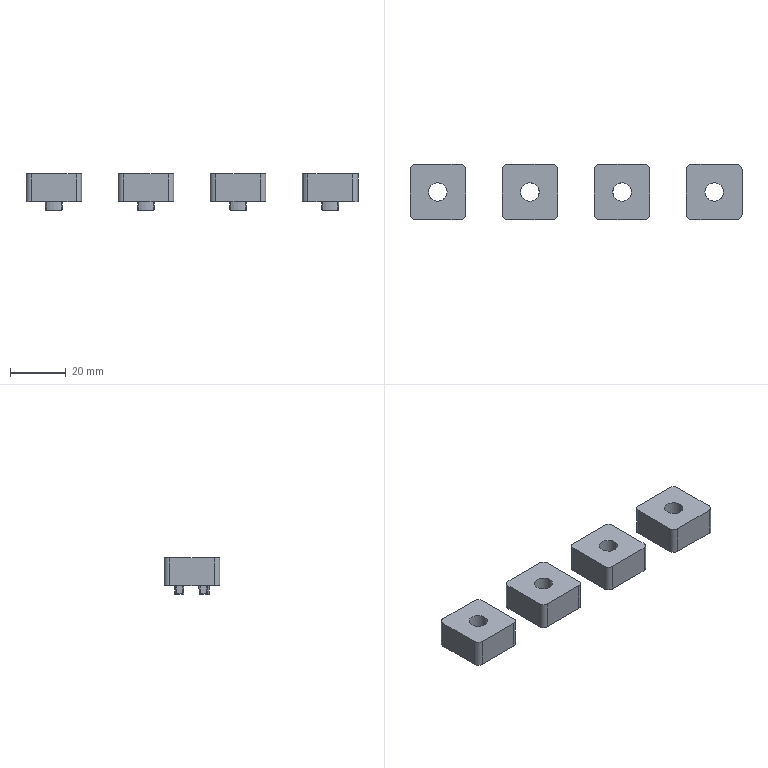NC program | NX | posted with a generic post | part box 118.91 x 19.91 x 13 mm
Lines 19 to 871 of 17620:
(ZLEVEL_PROFILE , TOOL : D10)
N36 T15 M6
N38 G54
N40 G17 G0 G90 X34.445 Y6.508 S9500 M3
N42 G43 Z30. H15
N44 Z1.5
N46 G94 G1 Y8.651 Z1.388 F1000.
N48 X34.782 Y10.25 Z1.302
N50 X35.476 Y11.729 Z1.216
N52 X36.49 Y13.01 Z1.131
N54 X37.771 Y14.024 Z1.045
N56 X39.25 Y14.718 Z0.96
N58 X40.849 Y15.055 Z0.874
N60 X58.151 Z-0.033
N62 X59.75 Y14.718 Z-0.118
N64 X61.229 Y14.024 Z-0.204
N66 X62.51 Y13.01 Z-0.29
N68 X63.524 Y11.729 Z-0.375
N70 X64.218 Y10.25 Z-0.461
N72 X64.555 Y8.651 Z-0.547
N74 Y0. Z-1.
N76 Y-8. F3000.
N78 G2 X57.5 Y-15.055 R7.055
N80 G1 X41.5
N82 G2 X34.445 Y-8. R7.055
N84 G1 Y8.
N86 G2 X41.5 Y15.055 R7.055
N88 G1 X57.5
N90 G2 X64.555 Y8. R7.055
N92 G1 Y0.
N94 Y-8. Z-1.074
N96 X64.528 Y-8.615 Z-1.08
N98 X64.448 Y-9.225 Z-1.085
N100 X64.315 Y-9.826 Z-1.091
N102 X64.13 Y-10.413 Z-1.097
N104 X63.894 Y-10.982 Z-1.102
N106 X63.61 Y-11.528 Z-1.108
N108 X63.279 Y-12.047 Z-1.114
N110 X62.904 Y-12.535 Z-1.119
N112 X62.489 Y-12.989 Z-1.125
N114 X62.035 Y-13.404 Z-1.131
N116 X61.547 Y-13.779 Z-1.136
N118 X61.028 Y-14.11 Z-1.142
N120 X60.482 Y-14.394 Z-1.148
N122 X59.913 Y-14.63 Z-1.153
N124 X59.326 Y-14.815 Z-1.159
N126 X58.725 Y-14.948 Z-1.165
N128 X58.115 Y-15.028 Z-1.17
N130 X57.5 Y-15.055 Z-1.176
N132 X41.5 Z-1.324
N134 X40.885 Y-15.028 Z-1.33
N136 X40.275 Y-14.948 Z-1.335
N138 X39.674 Y-14.815 Z-1.341
N140 X39.087 Y-14.63 Z-1.347
N142 X38.518 Y-14.394 Z-1.352
N144 X37.973 Y-14.11 Z-1.358
N146 X37.453 Y-13.779 Z-1.364
N148 X36.965 Y-13.404 Z-1.369
N150 X36.511 Y-12.989 Z-1.375
N152 X36.096 Y-12.535 Z-1.381
N154 X35.721 Y-12.047 Z-1.386
N156 X35.39 Y-11.528 Z-1.392
N158 X35.106 Y-10.982 Z-1.398
N160 X34.87 Y-10.413 Z-1.403
N162 X34.685 Y-9.826 Z-1.409
N164 X34.552 Y-9.225 Z-1.415
N166 X34.472 Y-8.615 Z-1.42
N168 X34.445 Y-8. Z-1.426
N170 Y0. Z-1.5
N172 Y4. Z-1.537
N174 Y8. Z-1.574
N176 X34.472 Y8.615 Z-1.58
N178 X34.552 Y9.225 Z-1.585
N180 X34.685 Y9.826 Z-1.591
N182 X34.87 Y10.413 Z-1.597
N184 X35.106 Y10.982 Z-1.602
N186 X35.39 Y11.528 Z-1.608
N188 X35.721 Y12.047 Z-1.614
N190 X36.096 Y12.535 Z-1.619
N192 X36.511 Y12.989 Z-1.625
N194 X36.965 Y13.404 Z-1.631
N196 X37.453 Y13.779 Z-1.636
N198 X37.973 Y14.11 Z-1.642
N200 X38.518 Y14.394 Z-1.648
N202 X39.087 Y14.63 Z-1.653
N204 X39.674 Y14.815 Z-1.659
N206 X40.275 Y14.948 Z-1.665
N208 X40.885 Y15.028 Z-1.67
N210 X41.5 Y15.055 Z-1.676
N212 X57.5 Z-1.824
N214 X58.115 Y15.028 Z-1.83
N216 X58.725 Y14.948 Z-1.835
N218 X59.326 Y14.815 Z-1.841
N220 X59.913 Y14.63 Z-1.847
N222 X60.482 Y14.394 Z-1.852
N224 X61.028 Y14.11 Z-1.858
N226 X61.547 Y13.779 Z-1.864
N228 X62.035 Y13.404 Z-1.869
N230 X62.489 Y12.989 Z-1.875
N232 X62.904 Y12.535 Z-1.881
N234 X63.279 Y12.047 Z-1.886
N236 X63.61 Y11.528 Z-1.892
N238 X63.894 Y10.982 Z-1.898
N240 X64.13 Y10.413 Z-1.903
N242 X64.315 Y9.826 Z-1.909
N244 X64.448 Y9.225 Z-1.915
N246 X64.528 Y8.615 Z-1.92
N248 X64.555 Y8. Z-1.926
N250 Y0. Z-2.
N252 Y-8. Z-2.074
N254 X64.528 Y-8.615 Z-2.08
N256 X64.448 Y-9.225 Z-2.085
N258 X64.315 Y-9.826 Z-2.091
N260 X64.13 Y-10.413 Z-2.097
N262 X63.894 Y-10.982 Z-2.102
N264 X63.61 Y-11.528 Z-2.108
N266 X63.279 Y-12.047 Z-2.114
N268 X62.904 Y-12.535 Z-2.119
N270 X62.489 Y-12.989 Z-2.125
N272 X62.035 Y-13.404 Z-2.131
N274 X61.547 Y-13.779 Z-2.136
N276 X61.028 Y-14.11 Z-2.142
N278 X60.482 Y-14.394 Z-2.148
N280 X59.913 Y-14.63 Z-2.153
N282 X59.326 Y-14.815 Z-2.159
N284 X58.725 Y-14.948 Z-2.165
N286 X58.115 Y-15.028 Z-2.17
N288 X57.5 Y-15.055 Z-2.176
N290 X41.5 Z-2.324
N292 X40.885 Y-15.028 Z-2.33
N294 X40.275 Y-14.948 Z-2.335
N296 X39.674 Y-14.815 Z-2.341
N298 X39.087 Y-14.63 Z-2.347
N300 X38.518 Y-14.394 Z-2.352
N302 X37.973 Y-14.11 Z-2.358
N304 X37.453 Y-13.779 Z-2.364
N306 X36.965 Y-13.404 Z-2.369
N308 X36.511 Y-12.989 Z-2.375
N310 X36.096 Y-12.535 Z-2.381
N312 X35.721 Y-12.047 Z-2.386
N314 X35.39 Y-11.528 Z-2.392
N316 X35.106 Y-10.982 Z-2.398
N318 X34.87 Y-10.413 Z-2.403
N320 X34.685 Y-9.826 Z-2.409
N322 X34.552 Y-9.225 Z-2.415
N324 X34.472 Y-8.615 Z-2.42
N326 X34.445 Y-8. Z-2.426
N328 Y0. Z-2.5
N330 Y4. Z-2.537
N332 Y8. Z-2.574
N334 X34.472 Y8.615 Z-2.58
N336 X34.552 Y9.225 Z-2.585
N338 X34.685 Y9.826 Z-2.591
N340 X34.87 Y10.413 Z-2.597
N342 X35.106 Y10.982 Z-2.602
N344 X35.39 Y11.528 Z-2.608
N346 X35.721 Y12.047 Z-2.614
N348 X36.096 Y12.535 Z-2.619
N350 X36.511 Y12.989 Z-2.625
N352 X36.965 Y13.404 Z-2.631
N354 X37.453 Y13.779 Z-2.636
N356 X37.973 Y14.11 Z-2.642
N358 X38.518 Y14.394 Z-2.648
N360 X39.087 Y14.63 Z-2.653
N362 X39.674 Y14.815 Z-2.659
N364 X40.275 Y14.948 Z-2.665
N366 X40.885 Y15.028 Z-2.67
N368 X41.5 Y15.055 Z-2.676
N370 X57.5 Z-2.824
N372 X58.115 Y15.028 Z-2.83
N374 X58.725 Y14.948 Z-2.835
N376 X59.326 Y14.815 Z-2.841
N378 X59.913 Y14.63 Z-2.847
N380 X60.482 Y14.394 Z-2.852
N382 X61.028 Y14.11 Z-2.858
N384 X61.547 Y13.779 Z-2.864
N386 X62.035 Y13.404 Z-2.869
N388 X62.489 Y12.989 Z-2.875
N390 X62.904 Y12.535 Z-2.881
N392 X63.279 Y12.047 Z-2.886
N394 X63.61 Y11.528 Z-2.892
N396 X63.894 Y10.982 Z-2.898
N398 X64.13 Y10.413 Z-2.903
N400 X64.315 Y9.826 Z-2.909
N402 X64.448 Y9.225 Z-2.915
N404 X64.528 Y8.615 Z-2.92
N406 X64.555 Y8. Z-2.926
N408 Y0. Z-3.
N410 Y-8. Z-3.074
N412 X64.528 Y-8.615 Z-3.08
N414 X64.448 Y-9.225 Z-3.085
N416 X64.315 Y-9.826 Z-3.091
N418 X64.13 Y-10.413 Z-3.097
N420 X63.894 Y-10.982 Z-3.102
N422 X63.61 Y-11.528 Z-3.108
N424 X63.279 Y-12.047 Z-3.114
N426 X62.904 Y-12.535 Z-3.119
N428 X62.489 Y-12.989 Z-3.125
N430 X62.035 Y-13.404 Z-3.131
N432 X61.547 Y-13.779 Z-3.136
N434 X61.028 Y-14.11 Z-3.142
N436 X60.482 Y-14.394 Z-3.148
N438 X59.913 Y-14.63 Z-3.153
N440 X59.326 Y-14.815 Z-3.159
N442 X58.725 Y-14.948 Z-3.165
N444 X58.115 Y-15.028 Z-3.17
N446 X57.5 Y-15.055 Z-3.176
N448 X41.5 Z-3.324
N450 X40.885 Y-15.028 Z-3.33
N452 X40.275 Y-14.948 Z-3.335
N454 X39.674 Y-14.815 Z-3.341
N456 X39.087 Y-14.63 Z-3.347
N458 X38.518 Y-14.394 Z-3.352
N460 X37.973 Y-14.11 Z-3.358
N462 X37.453 Y-13.779 Z-3.364
N464 X36.965 Y-13.404 Z-3.369
N466 X36.511 Y-12.989 Z-3.375
N468 X36.096 Y-12.535 Z-3.381
N470 X35.721 Y-12.047 Z-3.386
N472 X35.39 Y-11.528 Z-3.392
N474 X35.106 Y-10.982 Z-3.398
N476 X34.87 Y-10.413 Z-3.403
N478 X34.685 Y-9.826 Z-3.409
N480 X34.552 Y-9.225 Z-3.415
N482 X34.472 Y-8.615 Z-3.42
N484 X34.445 Y-8. Z-3.426
N486 Y0. Z-3.5
N488 Y4. Z-3.537
N490 Y8. Z-3.574
N492 X34.472 Y8.615 Z-3.58
N494 X34.552 Y9.225 Z-3.585
N496 X34.685 Y9.826 Z-3.591
N498 X34.87 Y10.413 Z-3.597
N500 X35.106 Y10.982 Z-3.602
N502 X35.39 Y11.528 Z-3.608
N504 X35.721 Y12.047 Z-3.614
N506 X36.096 Y12.535 Z-3.619
N508 X36.511 Y12.989 Z-3.625
N510 X36.965 Y13.404 Z-3.631
N512 X37.453 Y13.779 Z-3.636
N514 X37.973 Y14.11 Z-3.642
N516 X38.518 Y14.394 Z-3.648
N518 X39.087 Y14.63 Z-3.653
N520 X39.674 Y14.815 Z-3.659
N522 X40.275 Y14.948 Z-3.665
N524 X40.885 Y15.028 Z-3.67
N526 X41.5 Y15.055 Z-3.676
N528 X57.5 Z-3.824
N530 X58.115 Y15.028 Z-3.83
N532 X58.725 Y14.948 Z-3.835
N534 X59.326 Y14.815 Z-3.841
N536 X59.913 Y14.63 Z-3.847
N538 X60.482 Y14.394 Z-3.852
N540 X61.028 Y14.11 Z-3.858
N542 X61.547 Y13.779 Z-3.864
N544 X62.035 Y13.404 Z-3.869
N546 X62.489 Y12.989 Z-3.875
N548 X62.904 Y12.535 Z-3.881
N550 X63.279 Y12.047 Z-3.886
N552 X63.61 Y11.528 Z-3.892
N554 X63.894 Y10.982 Z-3.898
N556 X64.13 Y10.413 Z-3.903
N558 X64.315 Y9.826 Z-3.909
N560 X64.448 Y9.225 Z-3.915
N562 X64.528 Y8.615 Z-3.92
N564 X64.555 Y8. Z-3.926
N566 Y0. Z-4.
N568 Y-8. Z-4.074
N570 X64.528 Y-8.615 Z-4.08
N572 X64.448 Y-9.225 Z-4.085
N574 X64.315 Y-9.826 Z-4.091
N576 X64.13 Y-10.413 Z-4.097
N578 X63.894 Y-10.982 Z-4.102
N580 X63.61 Y-11.528 Z-4.108
N582 X63.279 Y-12.047 Z-4.114
N584 X62.904 Y-12.535 Z-4.119
N586 X62.489 Y-12.989 Z-4.125
N588 X62.035 Y-13.404 Z-4.131
N590 X61.547 Y-13.779 Z-4.136
N592 X61.028 Y-14.11 Z-4.142
N594 X60.482 Y-14.394 Z-4.148
N596 X59.913 Y-14.63 Z-4.153
N598 X59.326 Y-14.815 Z-4.159
N600 X58.725 Y-14.948 Z-4.165
N602 X58.115 Y-15.028 Z-4.17
N604 X57.5 Y-15.055 Z-4.176
N606 X41.5 Z-4.324
N608 X40.885 Y-15.028 Z-4.33
N610 X40.275 Y-14.948 Z-4.335
N612 X39.674 Y-14.815 Z-4.341
N614 X39.087 Y-14.63 Z-4.347
N616 X38.518 Y-14.394 Z-4.352
N618 X37.973 Y-14.11 Z-4.358
N620 X37.453 Y-13.779 Z-4.364
N622 X36.965 Y-13.404 Z-4.369
N624 X36.511 Y-12.989 Z-4.375
N626 X36.096 Y-12.535 Z-4.381
N628 X35.721 Y-12.047 Z-4.386
N630 X35.39 Y-11.528 Z-4.392
N632 X35.106 Y-10.982 Z-4.398
N634 X34.87 Y-10.413 Z-4.403
N636 X34.685 Y-9.826 Z-4.409
N638 X34.552 Y-9.225 Z-4.415
N640 X34.472 Y-8.615 Z-4.42
N642 X34.445 Y-8. Z-4.426
N644 Y0. Z-4.5
N646 Y4. Z-4.537
N648 Y8. Z-4.574
N650 X34.472 Y8.615 Z-4.58
N652 X34.552 Y9.225 Z-4.585
N654 X34.685 Y9.826 Z-4.591
N656 X34.87 Y10.413 Z-4.597
N658 X35.106 Y10.982 Z-4.602
N660 X35.39 Y11.528 Z-4.608
N662 X35.721 Y12.047 Z-4.614
N664 X36.096 Y12.535 Z-4.619
N666 X36.511 Y12.989 Z-4.625
N668 X36.965 Y13.404 Z-4.631
N670 X37.453 Y13.779 Z-4.636
N672 X37.973 Y14.11 Z-4.642
N674 X38.518 Y14.394 Z-4.648
N676 X39.087 Y14.63 Z-4.653
N678 X39.674 Y14.815 Z-4.659
N680 X40.275 Y14.948 Z-4.665
N682 X40.885 Y15.028 Z-4.67
N684 X41.5 Y15.055 Z-4.676
N686 X57.5 Z-4.824
N688 X58.115 Y15.028 Z-4.83
N690 X58.725 Y14.948 Z-4.835
N692 X59.326 Y14.815 Z-4.841
N694 X59.913 Y14.63 Z-4.847
N696 X60.482 Y14.394 Z-4.852
N698 X61.028 Y14.11 Z-4.858
N700 X61.547 Y13.779 Z-4.864
N702 X62.035 Y13.404 Z-4.869
N704 X62.489 Y12.989 Z-4.875
N706 X62.904 Y12.535 Z-4.881
N708 X63.279 Y12.047 Z-4.886
N710 X63.61 Y11.528 Z-4.892
N712 X63.894 Y10.982 Z-4.898
N714 X64.13 Y10.413 Z-4.903
N716 X64.315 Y9.826 Z-4.909
N718 X64.448 Y9.225 Z-4.915
N720 X64.528 Y8.615 Z-4.92
N722 X64.555 Y8. Z-4.926
N724 Y0. Z-5.
N726 Y-8. Z-5.074
N728 X64.528 Y-8.615 Z-5.08
N730 X64.448 Y-9.225 Z-5.085
N732 X64.315 Y-9.826 Z-5.091
N734 X64.13 Y-10.413 Z-5.097
N736 X63.894 Y-10.982 Z-5.102
N738 X63.61 Y-11.528 Z-5.108
N740 X63.279 Y-12.047 Z-5.114
N742 X62.904 Y-12.535 Z-5.119
N744 X62.489 Y-12.989 Z-5.125
N746 X62.035 Y-13.404 Z-5.131
N748 X61.547 Y-13.779 Z-5.136
N750 X61.028 Y-14.11 Z-5.142
N752 X60.482 Y-14.394 Z-5.148
N754 X59.913 Y-14.63 Z-5.153
N756 X59.326 Y-14.815 Z-5.159
N758 X58.725 Y-14.948 Z-5.165
N760 X58.115 Y-15.028 Z-5.17
N762 X57.5 Y-15.055 Z-5.176
N764 X41.5 Z-5.324
N766 X40.885 Y-15.028 Z-5.33
N768 X40.275 Y-14.948 Z-5.335
N770 X39.674 Y-14.815 Z-5.341
N772 X39.087 Y-14.63 Z-5.347
N774 X38.518 Y-14.394 Z-5.352
N776 X37.973 Y-14.11 Z-5.358
N778 X37.453 Y-13.779 Z-5.364
N780 X36.965 Y-13.404 Z-5.369
N782 X36.511 Y-12.989 Z-5.375
N784 X36.096 Y-12.535 Z-5.381
N786 X35.721 Y-12.047 Z-5.386
N788 X35.39 Y-11.528 Z-5.392
N790 X35.106 Y-10.982 Z-5.398
N792 X34.87 Y-10.413 Z-5.403
N794 X34.685 Y-9.826 Z-5.409
N796 X34.552 Y-9.225 Z-5.415
N798 X34.472 Y-8.615 Z-5.42
N800 X34.445 Y-8. Z-5.426
N802 Y0. Z-5.5
N804 Y4. Z-5.537
N806 Y8. Z-5.574
N808 X34.472 Y8.615 Z-5.58
N810 X34.552 Y9.225 Z-5.585
N812 X34.685 Y9.826 Z-5.591
N814 X34.87 Y10.413 Z-5.597
N816 X35.106 Y10.982 Z-5.602
N818 X35.39 Y11.528 Z-5.608
N820 X35.721 Y12.047 Z-5.614
N822 X36.096 Y12.535 Z-5.619
N824 X36.511 Y12.989 Z-5.625
N826 X36.965 Y13.404 Z-5.631
N828 X37.453 Y13.779 Z-5.636
N830 X37.973 Y14.11 Z-5.642
N832 X38.518 Y14.394 Z-5.648
N834 X39.087 Y14.63 Z-5.653
N836 X39.674 Y14.815 Z-5.659
N838 X40.275 Y14.948 Z-5.665
N840 X40.885 Y15.028 Z-5.67
N842 X41.5 Y15.055 Z-5.676
N844 X57.5 Z-5.824
N846 X58.115 Y15.028 Z-5.83
N848 X58.725 Y14.948 Z-5.835
N850 X59.326 Y14.815 Z-5.841
N852 X59.913 Y14.63 Z-5.847
N854 X60.482 Y14.394 Z-5.852
N856 X61.028 Y14.11 Z-5.858
N858 X61.547 Y13.779 Z-5.864
N860 X62.035 Y13.404 Z-5.869
N862 X62.489 Y12.989 Z-5.875
N864 X62.904 Y12.535 Z-5.881
N866 X63.279 Y12.047 Z-5.886
N868 X63.61 Y11.528 Z-5.892
N870 X63.894 Y10.982 Z-5.898
N872 X64.13 Y10.413 Z-5.903
N874 X64.315 Y9.826 Z-5.909
N876 X64.448 Y9.225 Z-5.915
N878 X64.528 Y8.615 Z-5.92
N880 X64.555 Y8. Z-5.926
N882 Y0. Z-6.
N884 Y-8. Z-6.074
N886 X64.528 Y-8.615 Z-6.08
N888 X64.448 Y-9.225 Z-6.085
N890 X64.315 Y-9.826 Z-6.091
N892 X64.13 Y-10.413 Z-6.097
N894 X63.894 Y-10.982 Z-6.102
N896 X63.61 Y-11.528 Z-6.108
N898 X63.279 Y-12.047 Z-6.114
N900 X62.904 Y-12.535 Z-6.119
N902 X62.489 Y-12.989 Z-6.125
N904 X62.035 Y-13.404 Z-6.131
N906 X61.547 Y-13.779 Z-6.136
N908 X61.028 Y-14.11 Z-6.142
N910 X60.482 Y-14.394 Z-6.148
N912 X59.913 Y-14.63 Z-6.153
N914 X59.326 Y-14.815 Z-6.159
N916 X58.725 Y-14.948 Z-6.165
N918 X58.115 Y-15.028 Z-6.17
N920 X57.5 Y-15.055 Z-6.176
N922 X41.5 Z-6.324
N924 X40.885 Y-15.028 Z-6.33
N926 X40.275 Y-14.948 Z-6.335
N928 X39.674 Y-14.815 Z-6.341
N930 X39.087 Y-14.63 Z-6.347
N932 X38.518 Y-14.394 Z-6.352
N934 X37.973 Y-14.11 Z-6.358
N936 X37.453 Y-13.779 Z-6.364
N938 X36.965 Y-13.404 Z-6.369
N940 X36.511 Y-12.989 Z-6.375
N942 X36.096 Y-12.535 Z-6.381
N944 X35.721 Y-12.047 Z-6.386
N946 X35.39 Y-11.528 Z-6.392
N948 X35.106 Y-10.982 Z-6.398
N950 X34.87 Y-10.413 Z-6.403
N952 X34.685 Y-9.826 Z-6.409
N954 X34.552 Y-9.225 Z-6.415
N956 X34.472 Y-8.615 Z-6.42
N958 X34.445 Y-8. Z-6.426
N960 Y0. Z-6.5
N962 Y4. Z-6.537
N964 Y8. Z-6.574
N966 X34.472 Y8.615 Z-6.58
N968 X34.552 Y9.225 Z-6.585
N970 X34.685 Y9.826 Z-6.591
N972 X34.87 Y10.413 Z-6.597
N974 X35.106 Y10.982 Z-6.602
N976 X35.39 Y11.528 Z-6.608
N978 X35.721 Y12.047 Z-6.614
N980 X36.096 Y12.535 Z-6.619
N982 X36.511 Y12.989 Z-6.625
N984 X36.965 Y13.404 Z-6.631
N986 X37.453 Y13.779 Z-6.636
N988 X37.973 Y14.11 Z-6.642
N990 X38.518 Y14.394 Z-6.648
N992 X39.087 Y14.63 Z-6.653
N994 X39.674 Y14.815 Z-6.659
N996 X40.275 Y14.948 Z-6.665
N998 X40.885 Y15.028 Z-6.67
N1000 X41.5 Y15.055 Z-6.676
N1002 X57.5 Z-6.824
N1004 X58.115 Y15.028 Z-6.83
N1006 X58.725 Y14.948 Z-6.835
N1008 X59.326 Y14.815 Z-6.841
N1010 X59.913 Y14.63 Z-6.847
N1012 X60.482 Y14.394 Z-6.852
N1014 X61.028 Y14.11 Z-6.858
N1016 X61.547 Y13.779 Z-6.864
N1018 X62.035 Y13.404 Z-6.869
N1020 X62.489 Y12.989 Z-6.875
N1022 X62.904 Y12.535 Z-6.881
N1024 X63.279 Y12.047 Z-6.886
N1026 X63.61 Y11.528 Z-6.892
N1028 X63.894 Y10.982 Z-6.898
N1030 X64.13 Y10.413 Z-6.903
N1032 X64.315 Y9.826 Z-6.909
N1034 X64.448 Y9.225 Z-6.915
N1036 X64.528 Y8.615 Z-6.92
N1038 X64.555 Y8. Z-6.926
N1040 Y0. Z-7.
N1042 Y-8. Z-7.074
N1044 X64.528 Y-8.615 Z-7.08
N1046 X64.448 Y-9.225 Z-7.085
N1048 X64.315 Y-9.826 Z-7.091
N1050 X64.13 Y-10.413 Z-7.097
N1052 X63.894 Y-10.982 Z-7.102
N1054 X63.61 Y-11.528 Z-7.108
N1056 X63.279 Y-12.047 Z-7.114
N1058 X62.904 Y-12.535 Z-7.119
N1060 X62.489 Y-12.989 Z-7.125
N1062 X62.035 Y-13.404 Z-7.131
N1064 X61.547 Y-13.779 Z-7.136
N1066 X61.028 Y-14.11 Z-7.142
N1068 X60.482 Y-14.394 Z-7.148
N1070 X59.913 Y-14.63 Z-7.153
N1072 X59.326 Y-14.815 Z-7.159
N1074 X58.725 Y-14.948 Z-7.165
N1076 X58.115 Y-15.028 Z-7.17
N1078 X57.5 Y-15.055 Z-7.176
N1080 X41.5 Z-7.324
N1082 X40.885 Y-15.028 Z-7.33
N1084 X40.275 Y-14.948 Z-7.335
N1086 X39.674 Y-14.815 Z-7.341
N1088 X39.087 Y-14.63 Z-7.347
N1090 X38.518 Y-14.394 Z-7.352
N1092 X37.973 Y-14.11 Z-7.358
N1094 X37.453 Y-13.779 Z-7.364
N1096 X36.965 Y-13.404 Z-7.369
N1098 X36.511 Y-12.989 Z-7.375
N1100 X36.096 Y-12.535 Z-7.381
N1102 X35.721 Y-12.047 Z-7.386
N1104 X35.39 Y-11.528 Z-7.392
N1106 X35.106 Y-10.982 Z-7.398
N1108 X34.87 Y-10.413 Z-7.403
N1110 X34.685 Y-9.826 Z-7.409
N1112 X34.552 Y-9.225 Z-7.415
N1114 X34.472 Y-8.615 Z-7.42
N1116 X34.445 Y-8. Z-7.426
N1118 Y0. Z-7.5
N1120 Y4. Z-7.537
N1122 Y8. Z-7.574
N1124 X34.472 Y8.615 Z-7.58
N1126 X34.552 Y9.225 Z-7.585
N1128 X34.685 Y9.826 Z-7.591
N1130 X34.87 Y10.413 Z-7.597
N1132 X35.106 Y10.982 Z-7.602
N1134 X35.39 Y11.528 Z-7.608
N1136 X35.721 Y12.047 Z-7.614
N1138 X36.096 Y12.535 Z-7.619
N1140 X36.511 Y12.989 Z-7.625
N1142 X36.965 Y13.404 Z-7.631
N1144 X37.453 Y13.779 Z-7.636
N1146 X37.973 Y14.11 Z-7.642
N1148 X38.518 Y14.394 Z-7.648
N1150 X39.087 Y14.63 Z-7.653
N1152 X39.674 Y14.815 Z-7.659
N1154 X40.275 Y14.948 Z-7.665
N1156 X40.885 Y15.028 Z-7.67
N1158 X41.5 Y15.055 Z-7.676
N1160 X57.5 Z-7.824
N1162 X58.115 Y15.028 Z-7.83
N1164 X58.725 Y14.948 Z-7.835
N1166 X59.326 Y14.815 Z-7.841
N1168 X59.913 Y14.63 Z-7.847
N1170 X60.482 Y14.394 Z-7.852
N1172 X61.028 Y14.11 Z-7.858
N1174 X61.547 Y13.779 Z-7.864
N1176 X62.035 Y13.404 Z-7.869
N1178 X62.489 Y12.989 Z-7.875
N1180 X62.904 Y12.535 Z-7.881
N1182 X63.279 Y12.047 Z-7.886
N1184 X63.61 Y11.528 Z-7.892
N1186 X63.894 Y10.982 Z-7.898
N1188 X64.13 Y10.413 Z-7.903
N1190 X64.315 Y9.826 Z-7.909
N1192 X64.448 Y9.225 Z-7.915
N1194 X64.528 Y8.615 Z-7.92
N1196 X64.555 Y8. Z-7.926
N1198 Y0. Z-8.
N1200 Y-8. Z-8.074
N1202 X64.528 Y-8.615 Z-8.08
N1204 X64.448 Y-9.225 Z-8.085
N1206 X64.315 Y-9.826 Z-8.091
N1208 X64.13 Y-10.413 Z-8.097
N1210 X63.894 Y-10.982 Z-8.102
N1212 X63.61 Y-11.528 Z-8.108
N1214 X63.279 Y-12.047 Z-8.114
N1216 X62.904 Y-12.535 Z-8.119
N1218 X62.489 Y-12.989 Z-8.125
N1220 X62.035 Y-13.404 Z-8.131
N1222 X61.547 Y-13.779 Z-8.136
N1224 X61.028 Y-14.11 Z-8.142
N1226 X60.482 Y-14.394 Z-8.148
N1228 X59.913 Y-14.63 Z-8.153
N1230 X59.326 Y-14.815 Z-8.159
N1232 X58.725 Y-14.948 Z-8.165
N1234 X58.115 Y-15.028 Z-8.17
N1236 X57.5 Y-15.055 Z-8.176
N1238 X41.5 Z-8.324
N1240 X40.885 Y-15.028 Z-8.33
N1242 X40.275 Y-14.948 Z-8.335
N1244 X39.674 Y-14.815 Z-8.341
N1246 X39.087 Y-14.63 Z-8.347
N1248 X38.518 Y-14.394 Z-8.352
N1250 X37.973 Y-14.11 Z-8.358
N1252 X37.453 Y-13.779 Z-8.364
N1254 X36.965 Y-13.404 Z-8.369
N1256 X36.511 Y-12.989 Z-8.375
N1258 X36.096 Y-12.535 Z-8.381
N1260 X35.721 Y-12.047 Z-8.386
N1262 X35.39 Y-11.528 Z-8.392
N1264 X35.106 Y-10.982 Z-8.398
N1266 X34.87 Y-10.413 Z-8.403
N1268 X34.685 Y-9.826 Z-8.409
N1270 X34.552 Y-9.225 Z-8.415
N1272 X34.472 Y-8.615 Z-8.42
N1274 X34.445 Y-8. Z-8.426
N1276 Y0. Z-8.5
N1278 Y4. Z-8.537
N1280 Y8. Z-8.574
N1282 X34.472 Y8.615 Z-8.58
N1284 X34.552 Y9.225 Z-8.585
N1286 X34.685 Y9.826 Z-8.591
N1288 X34.87 Y10.413 Z-8.597
N1290 X35.106 Y10.982 Z-8.602
N1292 X35.39 Y11.528 Z-8.608
N1294 X35.721 Y12.047 Z-8.614
N1296 X36.096 Y12.535 Z-8.619
N1298 X36.511 Y12.989 Z-8.625
N1300 X36.965 Y13.404 Z-8.631
N1302 X37.453 Y13.779 Z-8.636
N1304 X37.973 Y14.11 Z-8.642
N1306 X38.518 Y14.394 Z-8.648
N1308 X39.087 Y14.63 Z-8.653
N1310 X39.674 Y14.815 Z-8.659
N1312 X40.275 Y14.948 Z-8.665
N1314 X40.885 Y15.028 Z-8.67
N1316 X41.5 Y15.055 Z-8.676
N1318 X57.5 Z-8.824
N1320 X58.115 Y15.028 Z-8.83
N1322 X58.725 Y14.948 Z-8.835
N1324 X59.326 Y14.815 Z-8.841
N1326 X59.913 Y14.63 Z-8.847
N1328 X60.482 Y14.394 Z-8.852
N1330 X61.028 Y14.11 Z-8.858
N1332 X61.547 Y13.779 Z-8.864
N1334 X62.035 Y13.404 Z-8.869
N1336 X62.489 Y12.989 Z-8.875
N1338 X62.904 Y12.535 Z-8.881
N1340 X63.279 Y12.047 Z-8.886
N1342 X63.61 Y11.528 Z-8.892
N1344 X63.894 Y10.982 Z-8.898
N1346 X64.13 Y10.413 Z-8.903
N1348 X64.315 Y9.826 Z-8.909
N1350 X64.448 Y9.225 Z-8.915
N1352 X64.528 Y8.615 Z-8.92
N1354 X64.555 Y8. Z-8.926
N1356 Y0. Z-9.
N1358 Y-8. Z-9.074
N1360 X64.528 Y-8.615 Z-9.08
N1362 X64.448 Y-9.225 Z-9.085
N1364 X64.315 Y-9.826 Z-9.091
N1366 X64.13 Y-10.413 Z-9.097
N1368 X63.894 Y-10.982 Z-9.102
N1370 X63.61 Y-11.528 Z-9.108
N1372 X63.279 Y-12.047 Z-9.114
N1374 X62.904 Y-12.535 Z-9.119
N1376 X62.489 Y-12.989 Z-9.125
N1378 X62.035 Y-13.404 Z-9.131
N1380 X61.547 Y-13.779 Z-9.136
N1382 X61.028 Y-14.11 Z-9.142
N1384 X60.482 Y-14.394 Z-9.148
N1386 X59.913 Y-14.63 Z-9.153
N1388 X59.326 Y-14.815 Z-9.159
N1390 X58.725 Y-14.948 Z-9.165
N1392 X58.115 Y-15.028 Z-9.17
N1394 X57.5 Y-15.055 Z-9.176
N1396 X41.5 Z-9.324
N1398 X40.885 Y-15.028 Z-9.33
N1400 X40.275 Y-14.948 Z-9.335
N1402 X39.674 Y-14.815 Z-9.341
N1404 X39.087 Y-14.63 Z-9.347
N1406 X38.518 Y-14.394 Z-9.352
N1408 X37.973 Y-14.11 Z-9.358
N1410 X37.453 Y-13.779 Z-9.364
N1412 X36.965 Y-13.404 Z-9.369
N1414 X36.511 Y-12.989 Z-9.375
N1416 X36.096 Y-12.535 Z-9.381
N1418 X35.721 Y-12.047 Z-9.386
N1420 X35.39 Y-11.528 Z-9.392
N1422 X35.106 Y-10.982 Z-9.398
N1424 X34.87 Y-10.413 Z-9.403
N1426 X34.685 Y-9.826 Z-9.409
N1428 X34.552 Y-9.225 Z-9.415
N1430 X34.472 Y-8.615 Z-9.42
N1432 X34.445 Y-8. Z-9.426
N1434 Y0. Z-9.5
N1436 Y4. Z-9.537
N1438 Y8. Z-9.574
N1440 X34.472 Y8.615 Z-9.58
N1442 X34.552 Y9.225 Z-9.585
N1444 X34.685 Y9.826 Z-9.591
N1446 X34.87 Y10.413 Z-9.597
N1448 X35.106 Y10.982 Z-9.602
N1450 X35.39 Y11.528 Z-9.608
N1452 X35.721 Y12.047 Z-9.614
N1454 X36.096 Y12.535 Z-9.619
N1456 X36.511 Y12.989 Z-9.625
N1458 X36.965 Y13.404 Z-9.631
N1460 X37.453 Y13.779 Z-9.636
N1462 X37.973 Y14.11 Z-9.642
N1464 X38.518 Y14.394 Z-9.648
N1466 X39.087 Y14.63 Z-9.653
N1468 X39.674 Y14.815 Z-9.659
N1470 X40.275 Y14.948 Z-9.665
N1472 X40.885 Y15.028 Z-9.67
N1474 X41.5 Y15.055 Z-9.676
N1476 X57.5 Z-9.824
N1478 X58.115 Y15.028 Z-9.83
N1480 X58.725 Y14.948 Z-9.835
N1482 X59.326 Y14.815 Z-9.841
N1484 X59.913 Y14.63 Z-9.847
N1486 X60.482 Y14.394 Z-9.852
N1488 X61.028 Y14.11 Z-9.858
N1490 X61.547 Y13.779 Z-9.864
N1492 X62.035 Y13.404 Z-9.869
N1494 X62.489 Y12.989 Z-9.875
N1496 X62.904 Y12.535 Z-9.881
N1498 X63.279 Y12.047 Z-9.886
N1500 X63.61 Y11.528 Z-9.892
N1502 X63.894 Y10.982 Z-9.898
N1504 X64.13 Y10.413 Z-9.903
N1506 X64.315 Y9.826 Z-9.909
N1508 X64.448 Y9.225 Z-9.915
N1510 X64.528 Y8.615 Z-9.92
N1512 X64.555 Y8. Z-9.926
N1514 Y0. Z-10.
N1516 Y-8. Z-10.074
N1518 X64.528 Y-8.615 Z-10.08
N1520 X64.448 Y-9.225 Z-10.085
N1522 X64.315 Y-9.826 Z-10.091
N1524 X64.13 Y-10.413 Z-10.097
N1526 X63.894 Y-10.982 Z-10.102
N1528 X63.61 Y-11.528 Z-10.108
N1530 X63.279 Y-12.047 Z-10.114
N1532 X62.904 Y-12.535 Z-10.119
N1534 X62.489 Y-12.989 Z-10.125
N1536 X62.035 Y-13.404 Z-10.131
N1538 X61.547 Y-13.779 Z-10.136
N1540 X61.028 Y-14.11 Z-10.142
N1542 X60.482 Y-14.394 Z-10.148
N1544 X59.913 Y-14.63 Z-10.153
N1546 X59.326 Y-14.815 Z-10.159
N1548 X58.725 Y-14.948 Z-10.165
N1550 X58.115 Y-15.028 Z-10.17
N1552 X57.5 Y-15.055 Z-10.176
N1554 X41.5 Z-10.324
N1556 X40.885 Y-15.028 Z-10.33
N1558 X40.275 Y-14.948 Z-10.335
N1560 X39.674 Y-14.815 Z-10.341
N1562 X39.087 Y-14.63 Z-10.347
N1564 X38.518 Y-14.394 Z-10.352
N1566 X37.973 Y-14.11 Z-10.358
N1568 X37.453 Y-13.779 Z-10.364
N1570 X36.965 Y-13.404 Z-10.369
N1572 X36.511 Y-12.989 Z-10.375
N1574 X36.096 Y-12.535 Z-10.381
N1576 X35.721 Y-12.047 Z-10.386
N1578 X35.39 Y-11.528 Z-10.392
N1580 X35.106 Y-10.982 Z-10.398
N1582 X34.87 Y-10.413 Z-10.403
N1584 X34.685 Y-9.826 Z-10.409
N1586 X34.552 Y-9.225 Z-10.415
N1588 X34.472 Y-8.615 Z-10.42
N1590 X34.445 Y-8. Z-10.426
N1592 Y0. Z-10.5
N1594 Y4. Z-10.537
N1596 Y8. Z-10.574
N1598 X34.472 Y8.615 Z-10.58
N1600 X34.552 Y9.225 Z-10.585
N1602 X34.685 Y9.826 Z-10.591
N1604 X34.87 Y10.413 Z-10.597
N1606 X35.106 Y10.982 Z-10.602
N1608 X35.39 Y11.528 Z-10.608
N1610 X35.721 Y12.047 Z-10.614
N1612 X36.096 Y12.535 Z-10.619
N1614 X36.511 Y12.989 Z-10.625
N1616 X36.965 Y13.404 Z-10.631
N1618 X37.453 Y13.779 Z-10.636
N1620 X37.973 Y14.11 Z-10.642
N1622 X38.518 Y14.394 Z-10.648
N1624 X39.087 Y14.63 Z-10.653
N1626 X39.674 Y14.815 Z-10.659
N1628 X40.275 Y14.948 Z-10.665
N1630 X40.885 Y15.028 Z-10.67
N1632 X41.5 Y15.055 Z-10.676
N1634 X57.5 Z-10.824
N1636 X58.115 Y15.028 Z-10.83
N1638 X58.725 Y14.948 Z-10.835
N1640 X59.326 Y14.815 Z-10.841
N1642 X59.913 Y14.63 Z-10.847
N1644 X60.482 Y14.394 Z-10.852
N1646 X61.028 Y14.11 Z-10.858
N1648 X61.547 Y13.779 Z-10.864
N1650 X62.035 Y13.404 Z-10.869
N1652 X62.489 Y12.989 Z-10.875
N1654 X62.904 Y12.535 Z-10.881
N1656 X63.279 Y12.047 Z-10.886
N1658 X63.61 Y11.528 Z-10.892
N1660 X63.894 Y10.982 Z-10.898
N1662 X64.13 Y10.413 Z-10.903
N1664 X64.315 Y9.826 Z-10.909
N1666 X64.448 Y9.225 Z-10.915
N1668 X64.528 Y8.615 Z-10.92
N1670 X64.555 Y8. Z-10.926
N1672 Y0. Z-11.
N1674 Y-8. Z-11.074
N1676 X64.528 Y-8.615 Z-11.08
N1678 X64.448 Y-9.225 Z-11.085
N1680 X64.315 Y-9.826 Z-11.091
N1682 X64.13 Y-10.413 Z-11.097
N1684 X63.894 Y-10.982 Z-11.102
N1686 X63.61 Y-11.528 Z-11.108
N1688 X63.279 Y-12.047 Z-11.114
N1690 X62.904 Y-12.535 Z-11.119
N1692 X62.489 Y-12.989 Z-11.125
N1694 X62.035 Y-13.404 Z-11.131
N1696 X61.547 Y-13.779 Z-11.136
N1698 X61.028 Y-14.11 Z-11.142
N1700 X60.482 Y-14.394 Z-11.148
N1702 X59.913 Y-14.63 Z-11.153
N1704 X59.326 Y-14.815 Z-11.159
N1706 X58.725 Y-14.948 Z-11.165
N1708 X58.115 Y-15.028 Z-11.17
N1710 X57.5 Y-15.055 Z-11.176
N1712 X41.5 Z-11.324
N1714 X40.885 Y-15.028 Z-11.33
N1716 X40.275 Y-14.948 Z-11.335
N1718 X39.674 Y-14.815 Z-11.341
N1720 X39.087 Y-14.63 Z-11.347
N1722 X38.518 Y-14.394 Z-11.352
N1724 X37.973 Y-14.11 Z-11.358
N1726 X37.453 Y-13.779 Z-11.364
N1728 X36.965 Y-13.404 Z-11.369
N1730 X36.511 Y-12.989 Z-11.375
N1732 X36.096 Y-12.535 Z-11.381
N1734 X35.721 Y-12.047 Z-11.386